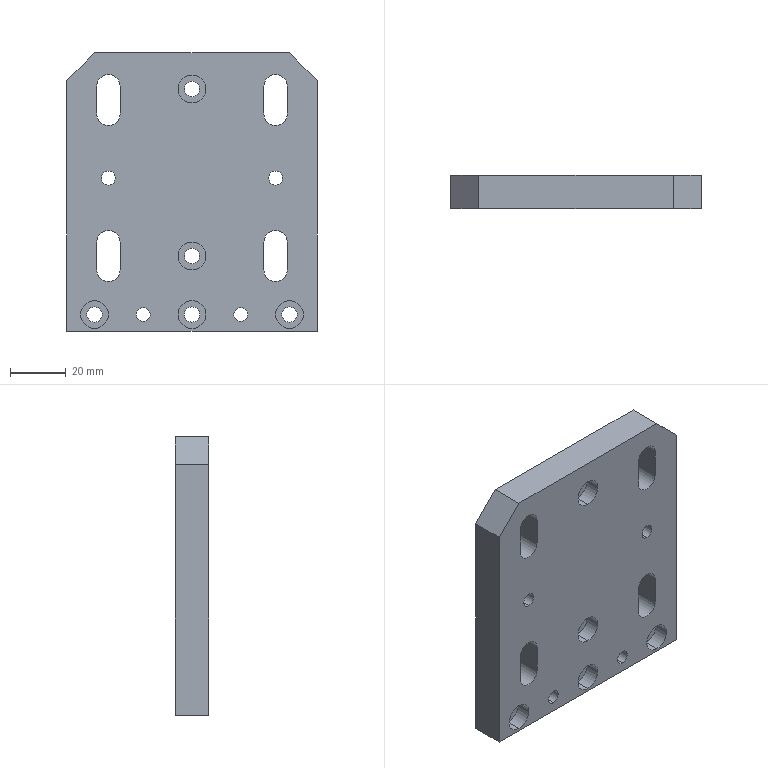Part | STEP file | PN_0012 | 1 solid | 61 faces | box 90 x 12 x 100 mm | volume 96261 mm3 | cylinder 40 | plane 21 | commonest cylinder face diameters 8.4 x12 5.5 x10 10 x10 5 x8